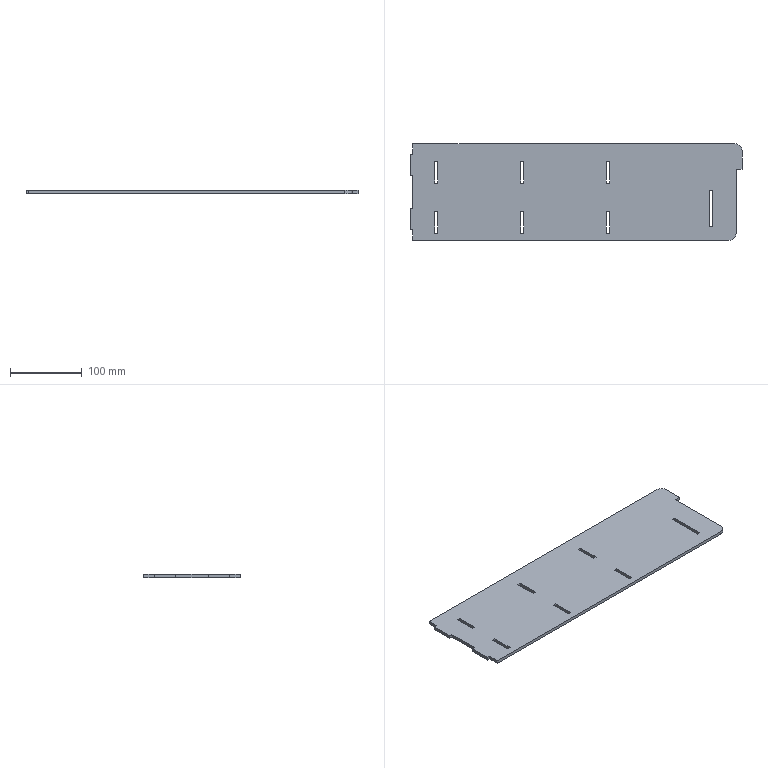Part | SolidWorks | features Fillet 1, FlatPattern 1, SMBaseFlange 1, SheetMetal 1 | 1 solid | 46 faces | box 464 x 135 x 4.5 mm | volume 271971 mm3 | plane 44 | cylinder 2 | commonest cylinder face diameters 20 x2
STEP:
#1=CARTESIAN_POINT('',(-230.,-90.,4.5));
#2=VERTEX_POINT('',#1);
#3=CARTESIAN_POINT('',(211.7,-90.,4.5));
#4=VERTEX_POINT('',#3);
#5=CARTESIAN_POINT('',(-230.,-90.,4.5));
#6=DIRECTION('',(1.,0.,0.));
#7=VECTOR('',#6,1000.);
#8=LINE('',#5,#7);
#9=EDGE_CURVE('',#2,#4,#8,.T.);
#10=ORIENTED_EDGE('',*,*,#9,.T.);
#11=CARTESIAN_POINT('',(221.7,-80.,4.5));
#12=VERTEX_POINT('',#11);
#13=CARTESIAN_POINT('',(211.7,-80.,4.5));
#14=DIRECTION('',(0.,0.,1.));
#15=DIRECTION('',(1.,0.,0.));
#16=AXIS2_PLACEMENT_3D('',#13,#14,#15);
#17=CIRCLE('',#16,10.);
#18=EDGE_CURVE('',#4,#12,#17,.T.);
#19=ORIENTED_EDGE('',*,*,#18,.T.);
#20=CARTESIAN_POINT('',(221.7,9.3,4.5));
#21=VERTEX_POINT('',#20);
#22=CARTESIAN_POINT('',(221.7,9.3,4.5));
#23=DIRECTION('',(0.,1.,0.));
#24=VECTOR('',#23,1000.);
#25=LINE('',#22,#24);
#26=EDGE_CURVE('',#12,#21,#25,.T.);
#27=ORIENTED_EDGE('',*,*,#26,.T.);
#28=CARTESIAN_POINT('',(230.,9.3,4.5));
#29=VERTEX_POINT('',#28);
#30=CARTESIAN_POINT('',(221.7,9.3,4.5));
#31=DIRECTION('',(1.,0.,0.));
#32=VECTOR('',#31,1000.);
#33=LINE('',#30,#32);
#34=EDGE_CURVE('',#21,#29,#33,.T.);
#35=ORIENTED_EDGE('',*,*,#34,.T.);
#36=CARTESIAN_POINT('',(230.,35.,4.5));
#37=VERTEX_POINT('',#36);
#38=CARTESIAN_POINT('',(230.,9.3,4.5));
#39=DIRECTION('',(0.,1.,0.));
#40=VECTOR('',#39,1000.);
#41=LINE('',#38,#40);
#42=EDGE_CURVE('',#29,#37,#41,.T.);
#43=ORIENTED_EDGE('',*,*,#42,.T.);
#44=CARTESIAN_POINT('',(220.,45.,4.5));
#45=VERTEX_POINT('',#44);
#46=CARTESIAN_POINT('',(220.,35.,4.5));
#47=DIRECTION('',(0.,0.,1.));
#48=DIRECTION('',(1.,0.,0.));
#49=AXIS2_PLACEMENT_3D('',#46,#47,#48);
#50=CIRCLE('',#49,10.);
#51=EDGE_CURVE('',#37,#45,#50,.T.);
#52=ORIENTED_EDGE('',*,*,#51,.T.);
#53=CARTESIAN_POINT('',(-230.,45.,4.5));
#54=VERTEX_POINT('',#53);
#55=CARTESIAN_POINT('',(-230.,45.,4.5));
#56=DIRECTION('',(-1.,0.,0.));
#57=VECTOR('',#56,1000.);
#58=LINE('',#55,#57);
#59=EDGE_CURVE('',#45,#54,#58,.T.);
#60=ORIENTED_EDGE('',*,*,#59,.T.);
#61=CARTESIAN_POINT('',(-230.,30.,4.5));
#62=VERTEX_POINT('',#61);
#63=CARTESIAN_POINT('',(-230.,45.,4.5));
#64=DIRECTION('',(0.,-1.,0.));
#65=VECTOR('',#64,1000.);
#66=LINE('',#63,#65);
#67=EDGE_CURVE('',#54,#62,#66,.T.);
#68=ORIENTED_EDGE('',*,*,#67,.T.);
#69=CARTESIAN_POINT('',(-234.,30.,4.5));
#70=VERTEX_POINT('',#69);
#71=CARTESIAN_POINT('',(-234.,30.,4.5));
#72=DIRECTION('',(-1.,0.,0.));
#73=VECTOR('',#72,1000.);
#74=LINE('',#71,#73);
#75=EDGE_CURVE('',#62,#70,#74,.T.);
#76=ORIENTED_EDGE('',*,*,#75,.T.);
#77=CARTESIAN_POINT('',(-234.,0.,4.5));
#78=VERTEX_POINT('',#77);
#79=CARTESIAN_POINT('',(-234.,0.,4.5));
#80=DIRECTION('',(0.,-1.,0.));
#81=VECTOR('',#80,1000.);
#82=LINE('',#79,#81);
#83=EDGE_CURVE('',#70,#78,#82,.T.);
#84=ORIENTED_EDGE('',*,*,#83,.T.);
#85=CARTESIAN_POINT('',(-230.,0.,4.5));
#86=VERTEX_POINT('',#85);
#87=CARTESIAN_POINT('',(-230.,0.,4.5));
#88=DIRECTION('',(1.,0.,0.));
#89=VECTOR('',#88,1000.);
#90=LINE('',#87,#89);
#91=EDGE_CURVE('',#78,#86,#90,.T.);
#92=ORIENTED_EDGE('',*,*,#91,.T.);
#93=CARTESIAN_POINT('',(-230.,-45.,4.5));
#94=VERTEX_POINT('',#93);
#95=CARTESIAN_POINT('',(-230.,0.,4.5));
#96=DIRECTION('',(0.,-1.,0.));
#97=VECTOR('',#96,1000.);
#98=LINE('',#95,#97);
#99=EDGE_CURVE('',#86,#94,#98,.T.);
#100=ORIENTED_EDGE('',*,*,#99,.T.);
#101=CARTESIAN_POINT('',(-234.,-45.,4.5));
#102=VERTEX_POINT('',#101);
#103=CARTESIAN_POINT('',(-234.,-45.,4.5));
#104=DIRECTION('',(-1.,0.,0.));
#105=VECTOR('',#104,1000.);
#106=LINE('',#103,#105);
#107=EDGE_CURVE('',#94,#102,#106,.T.);
#108=ORIENTED_EDGE('',*,*,#107,.T.);
#109=CARTESIAN_POINT('',(-234.,-75.,4.5));
#110=VERTEX_POINT('',#109);
#111=CARTESIAN_POINT('',(-234.,-75.,4.5));
#112=DIRECTION('',(0.,-1.,0.));
#113=VECTOR('',#112,1000.);
#114=LINE('',#111,#113);
#115=EDGE_CURVE('',#102,#110,#114,.T.);
#116=ORIENTED_EDGE('',*,*,#115,.T.);
#117=CARTESIAN_POINT('',(-230.,-75.,4.5));
#118=VERTEX_POINT('',#117);
#119=CARTESIAN_POINT('',(-230.,-75.,4.5));
#120=DIRECTION('',(1.,0.,0.));
#121=VECTOR('',#120,1000.);
#122=LINE('',#119,#121);
#123=EDGE_CURVE('',#110,#118,#122,.T.);
#124=ORIENTED_EDGE('',*,*,#123,.T.);
#125=CARTESIAN_POINT('',(-230.,-75.,4.5));
#126=DIRECTION('',(0.,-1.,0.));
#127=VECTOR('',#126,1000.);
#128=LINE('',#125,#127);
#129=EDGE_CURVE('',#118,#2,#128,.T.);
#130=ORIENTED_EDGE('',*,*,#129,.T.);
#131=EDGE_LOOP('',(#10,#19,#27,#35,#43,#52,#60,#68,#76,#84,#92,#100,#108,#116,#124,#130));
#132=FACE_OUTER_BOUND('',#131,.T.);
#133=CARTESIAN_POINT('',(189.,-20.7,4.5));
#134=VERTEX_POINT('',#133);
#135=CARTESIAN_POINT('',(184.5,-20.7,4.5));
#136=VERTEX_POINT('',#135);
#137=CARTESIAN_POINT('',(189.,-20.7,4.5));
#138=DIRECTION('',(-1.,0.,0.));
#139=VECTOR('',#138,1000.);
#140=LINE('',#137,#139);
#141=EDGE_CURVE('',#134,#136,#140,.T.);
#142=ORIENTED_EDGE('',*,*,#141,.F.);
#143=CARTESIAN_POINT('',(189.,-70.7,4.5));
#144=VERTEX_POINT('',#143);
#145=CARTESIAN_POINT('',(189.,-70.7,4.5));
#146=DIRECTION('',(0.,1.,0.));
#147=VECTOR('',#146,1000.);
#148=LINE('',#145,#147);
#149=EDGE_CURVE('',#144,#134,#148,.T.);
#150=ORIENTED_EDGE('',*,*,#149,.F.);
#151=CARTESIAN_POINT('',(184.5,-70.7,4.5));
#152=VERTEX_POINT('',#151);
#153=CARTESIAN_POINT('',(189.,-70.7,4.5));
#154=DIRECTION('',(1.,0.,0.));
#155=VECTOR('',#154,1000.);
#156=LINE('',#153,#155);
#157=EDGE_CURVE('',#152,#144,#156,.T.);
#158=ORIENTED_EDGE('',*,*,#157,.F.);
#159=CARTESIAN_POINT('',(184.5,-70.7,4.5));
#160=DIRECTION('',(0.,-1.,0.));
#161=VECTOR('',#160,1000.);
#162=LINE('',#159,#161);
#163=EDGE_CURVE('',#136,#152,#162,.T.);
#164=ORIENTED_EDGE('',*,*,#163,.F.);
#165=EDGE_LOOP('',(#142,#150,#158,#164));
#166=FACE_BOUND('',#165,.T.);
#167=CARTESIAN_POINT('',(45.,-50.,4.5));
#168=VERTEX_POINT('',#167);
#169=CARTESIAN_POINT('',(40.5,-50.,4.5));
#170=VERTEX_POINT('',#169);
#171=CARTESIAN_POINT('',(45.,-50.,4.5));
#172=DIRECTION('',(-1.,0.,0.));
#173=VECTOR('',#172,1000.);
#174=LINE('',#171,#173);
#175=EDGE_CURVE('',#168,#170,#174,.T.);
#176=ORIENTED_EDGE('',*,*,#175,.F.);
#177=CARTESIAN_POINT('',(45.,-80.,4.5));
#178=VERTEX_POINT('',#177);
#179=CARTESIAN_POINT('',(45.,-80.,4.5));
#180=DIRECTION('',(0.,1.,0.));
#181=VECTOR('',#180,1000.);
#182=LINE('',#179,#181);
#183=EDGE_CURVE('',#178,#168,#182,.T.);
#184=ORIENTED_EDGE('',*,*,#183,.F.);
#185=CARTESIAN_POINT('',(40.5,-80.,4.5));
#186=VERTEX_POINT('',#185);
#187=CARTESIAN_POINT('',(45.,-80.,4.5));
#188=DIRECTION('',(1.,0.,0.));
#189=VECTOR('',#188,1000.);
#190=LINE('',#187,#189);
#191=EDGE_CURVE('',#186,#178,#190,.T.);
#192=ORIENTED_EDGE('',*,*,#191,.F.);
#193=CARTESIAN_POINT('',(40.5,-80.,4.5));
#194=DIRECTION('',(0.,-1.,0.));
#195=VECTOR('',#194,1000.);
#196=LINE('',#193,#195);
#197=EDGE_CURVE('',#170,#186,#196,.T.);
#198=ORIENTED_EDGE('',*,*,#197,.F.);
#199=EDGE_LOOP('',(#176,#184,#192,#198));
#200=FACE_BOUND('',#199,.T.);
#201=CARTESIAN_POINT('',(45.,20.,4.5));
#202=VERTEX_POINT('',#201);
#203=CARTESIAN_POINT('',(40.5,20.,4.5));
#204=VERTEX_POINT('',#203);
#205=CARTESIAN_POINT('',(45.,20.,4.5));
#206=DIRECTION('',(-1.,0.,0.));
#207=VECTOR('',#206,1000.);
#208=LINE('',#205,#207);
#209=EDGE_CURVE('',#202,#204,#208,.T.);
#210=ORIENTED_EDGE('',*,*,#209,.F.);
#211=CARTESIAN_POINT('',(45.,-10.,4.5));
#212=VERTEX_POINT('',#211);
#213=CARTESIAN_POINT('',(45.,-10.,4.5));
#214=DIRECTION('',(0.,1.,0.));
#215=VECTOR('',#214,1000.);
#216=LINE('',#213,#215);
#217=EDGE_CURVE('',#212,#202,#216,.T.);
#218=ORIENTED_EDGE('',*,*,#217,.F.);
#219=CARTESIAN_POINT('',(40.5,-10.,4.5));
#220=VERTEX_POINT('',#219);
#221=CARTESIAN_POINT('',(45.,-10.,4.5));
#222=DIRECTION('',(1.,0.,0.));
#223=VECTOR('',#222,1000.);
#224=LINE('',#221,#223);
#225=EDGE_CURVE('',#220,#212,#224,.T.);
#226=ORIENTED_EDGE('',*,*,#225,.F.);
#227=CARTESIAN_POINT('',(40.5,-10.,4.5));
#228=DIRECTION('',(0.,-1.,0.));
#229=VECTOR('',#228,1000.);
#230=LINE('',#227,#229);
#231=EDGE_CURVE('',#204,#220,#230,.T.);
#232=ORIENTED_EDGE('',*,*,#231,.F.);
#233=EDGE_LOOP('',(#210,#218,#226,#232));
#234=FACE_BOUND('',#233,.T.);
#235=CARTESIAN_POINT('',(-75.,20.,4.5));
#236=VERTEX_POINT('',#235);
#237=CARTESIAN_POINT('',(-79.5,20.,4.5));
#238=VERTEX_POINT('',#237);
#239=CARTESIAN_POINT('',(-75.,20.,4.5));
#240=DIRECTION('',(-1.,0.,0.));
#241=VECTOR('',#240,1000.);
#242=LINE('',#239,#241);
#243=EDGE_CURVE('',#236,#238,#242,.T.);
#244=ORIENTED_EDGE('',*,*,#243,.F.);
#245=CARTESIAN_POINT('',(-75.,-10.,4.5));
#246=VERTEX_POINT('',#245);
#247=CARTESIAN_POINT('',(-75.,20.,4.5));
#248=DIRECTION('',(0.,1.,0.));
#249=VECTOR('',#248,1000.);
#250=LINE('',#247,#249);
#251=EDGE_CURVE('',#246,#236,#250,.T.);
#252=ORIENTED_EDGE('',*,*,#251,.F.);
#253=CARTESIAN_POINT('',(-79.5,-10.,4.5));
#254=VERTEX_POINT('',#253);
#255=CARTESIAN_POINT('',(-75.,-10.,4.5));
#256=DIRECTION('',(1.,0.,0.));
#257=VECTOR('',#256,1000.);
#258=LINE('',#255,#257);
#259=EDGE_CURVE('',#254,#246,#258,.T.);
#260=ORIENTED_EDGE('',*,*,#259,.F.);
#261=CARTESIAN_POINT('',(-79.5,20.,4.5));
#262=DIRECTION('',(0.,-1.,0.));
#263=VECTOR('',#262,1000.);
#264=LINE('',#261,#263);
#265=EDGE_CURVE('',#238,#254,#264,.T.);
#266=ORIENTED_EDGE('',*,*,#265,.F.);
#267=EDGE_LOOP('',(#244,#252,#260,#266));
#268=FACE_BOUND('',#267,.T.);
#269=CARTESIAN_POINT('',(-75.,-50.,4.5));
#270=VERTEX_POINT('',#269);
#271=CARTESIAN_POINT('',(-79.5,-50.,4.5));
#272=VERTEX_POINT('',#271);
#273=CARTESIAN_POINT('',(-75.,-50.,4.5));
#274=DIRECTION('',(-1.,0.,0.));
#275=VECTOR('',#274,1000.);
#276=LINE('',#273,#275);
#277=EDGE_CURVE('',#270,#272,#276,.T.);
#278=ORIENTED_EDGE('',*,*,#277,.F.);
#279=CARTESIAN_POINT('',(-75.,-80.,4.5));
#280=VERTEX_POINT('',#279);
#281=CARTESIAN_POINT('',(-75.,-80.,4.5));
#282=DIRECTION('',(0.,1.,0.));
#283=VECTOR('',#282,1000.);
#284=LINE('',#281,#283);
#285=EDGE_CURVE('',#280,#270,#284,.T.);
#286=ORIENTED_EDGE('',*,*,#285,.F.);
#287=CARTESIAN_POINT('',(-79.5,-80.,4.5));
#288=VERTEX_POINT('',#287);
#289=CARTESIAN_POINT('',(-75.,-80.,4.5));
#290=DIRECTION('',(1.,0.,0.));
#291=VECTOR('',#290,1000.);
#292=LINE('',#289,#291);
#293=EDGE_CURVE('',#288,#280,#292,.T.);
#294=ORIENTED_EDGE('',*,*,#293,.F.);
#295=CARTESIAN_POINT('',(-79.5,-80.,4.5));
#296=DIRECTION('',(0.,-1.,0.));
#297=VECTOR('',#296,1000.);
#298=LINE('',#295,#297);
#299=EDGE_CURVE('',#272,#288,#298,.T.);
#300=ORIENTED_EDGE('',*,*,#299,.F.);
#301=EDGE_LOOP('',(#278,#286,#294,#300));
#302=FACE_BOUND('',#301,.T.);
#303=CARTESIAN_POINT('',(-195.,20.,4.5));
#304=VERTEX_POINT('',#303);
#305=CARTESIAN_POINT('',(-199.5,20.,4.5));
#306=VERTEX_POINT('',#305);
#307=CARTESIAN_POINT('',(-195.,20.,4.5));
#308=DIRECTION('',(-1.,0.,0.));
#309=VECTOR('',#308,1000.);
#310=LINE('',#307,#309);
#311=EDGE_CURVE('',#304,#306,#310,.T.);
#312=ORIENTED_EDGE('',*,*,#311,.F.);
#313=CARTESIAN_POINT('',(-195.,-10.,4.5));
#314=VERTEX_POINT('',#313);
#315=CARTESIAN_POINT('',(-195.,20.,4.5));
#316=DIRECTION('',(0.,1.,0.));
#317=VECTOR('',#316,1000.);
#318=LINE('',#315,#317);
#319=EDGE_CURVE('',#314,#304,#318,.T.);
#320=ORIENTED_EDGE('',*,*,#319,.F.);
#321=CARTESIAN_POINT('',(-199.5,-10.,4.5));
#322=VERTEX_POINT('',#321);
#323=CARTESIAN_POINT('',(-195.,-10.,4.5));
#324=DIRECTION('',(1.,0.,0.));
#325=VECTOR('',#324,1000.);
#326=LINE('',#323,#325);
#327=EDGE_CURVE('',#322,#314,#326,.T.);
#328=ORIENTED_EDGE('',*,*,#327,.F.);
#329=CARTESIAN_POINT('',(-199.5,20.,4.5));
#330=DIRECTION('',(0.,-1.,0.));
#331=VECTOR('',#330,1000.);
#332=LINE('',#329,#331);
#333=EDGE_CURVE('',#306,#322,#332,.T.);
#334=ORIENTED_EDGE('',*,*,#333,.F.);
#335=EDGE_LOOP('',(#312,#320,#328,#334));
#336=FACE_BOUND('',#335,.T.);
#337=CARTESIAN_POINT('',(-195.,-50.,4.5));
#338=VERTEX_POINT('',#337);
#339=CARTESIAN_POINT('',(-199.5,-50.,4.5));
#340=VERTEX_POINT('',#339);
#341=CARTESIAN_POINT('',(-195.,-50.,4.5));
#342=DIRECTION('',(-1.,0.,0.));
#343=VECTOR('',#342,1000.);
#344=LINE('',#341,#343);
#345=EDGE_CURVE('',#338,#340,#344,.T.);
#346=ORIENTED_EDGE('',*,*,#345,.F.);
#347=CARTESIAN_POINT('',(-195.,-80.,4.5));
#348=VERTEX_POINT('',#347);
#349=CARTESIAN_POINT('',(-195.,-80.,4.5));
#350=DIRECTION('',(0.,1.,0.));
#351=VECTOR('',#350,1000.);
#352=LINE('',#349,#351);
#353=EDGE_CURVE('',#348,#338,#352,.T.);
#354=ORIENTED_EDGE('',*,*,#353,.F.);
#355=CARTESIAN_POINT('',(-199.5,-80.,4.5));
#356=VERTEX_POINT('',#355);
#357=CARTESIAN_POINT('',(-195.,-80.,4.5));
#358=DIRECTION('',(1.,0.,0.));
#359=VECTOR('',#358,1000.);
#360=LINE('',#357,#359);
#361=EDGE_CURVE('',#356,#348,#360,.T.);
#362=ORIENTED_EDGE('',*,*,#361,.F.);
#363=CARTESIAN_POINT('',(-199.5,-80.,4.5));
#364=DIRECTION('',(0.,-1.,0.));
#365=VECTOR('',#364,1000.);
#366=LINE('',#363,#365);
#367=EDGE_CURVE('',#340,#356,#366,.T.);
#368=ORIENTED_EDGE('',*,*,#367,.F.);
#369=EDGE_LOOP('',(#346,#354,#362,#368));
#370=FACE_BOUND('',#369,.T.);
#371=CARTESIAN_POINT('',(0.,0.,4.5));
#372=DIRECTION('',(0.,0.,1.));
#373=DIRECTION('',(1.,0.,0.));
#374=AXIS2_PLACEMENT_3D('',#371,#372,#373);
#375=PLANE('',#374);
#376=ADVANCED_FACE('',(#132,#166,#200,#234,#268,#302,#336,#370),#375,.T.);
#377=CARTESIAN_POINT('',(-195.,-10.,0.));
#378=VERTEX_POINT('',#377);
#379=CARTESIAN_POINT('',(-195.,20.,0.));
#380=VERTEX_POINT('',#379);
#381=CARTESIAN_POINT('',(-195.,20.,0.));
#382=DIRECTION('',(0.,1.,0.));
#383=VECTOR('',#382,1000.);
#384=LINE('',#381,#383);
#385=EDGE_CURVE('',#378,#380,#384,.T.);
#386=ORIENTED_EDGE('',*,*,#385,.T.);
#387=CARTESIAN_POINT('',(-199.5,20.,0.));
#388=VERTEX_POINT('',#387);
#389=CARTESIAN_POINT('',(-195.,20.,0.));
#390=DIRECTION('',(-1.,0.,0.));
#391=VECTOR('',#390,1000.);
#392=LINE('',#389,#391);
#393=EDGE_CURVE('',#380,#388,#392,.T.);
#394=ORIENTED_EDGE('',*,*,#393,.T.);
#395=CARTESIAN_POINT('',(-199.5,-10.,0.));
#396=VERTEX_POINT('',#395);
#397=CARTESIAN_POINT('',(-199.5,20.,0.));
#398=DIRECTION('',(0.,-1.,0.));
#399=VECTOR('',#398,1000.);
#400=LINE('',#397,#399);
#401=EDGE_CURVE('',#388,#396,#400,.T.);
#402=ORIENTED_EDGE('',*,*,#401,.T.);
#403=CARTESIAN_POINT('',(-195.,-10.,0.));
#404=DIRECTION('',(1.,0.,0.));
#405=VECTOR('',#404,1000.);
#406=LINE('',#403,#405);
#407=EDGE_CURVE('',#396,#378,#406,.T.);
#408=ORIENTED_EDGE('',*,*,#407,.T.);
#409=EDGE_LOOP('',(#386,#394,#402,#408));
#410=FACE_BOUND('',#409,.T.);
#411=CARTESIAN_POINT('',(-75.,-10.,0.));
#412=VERTEX_POINT('',#411);
#413=CARTESIAN_POINT('',(-75.,20.,0.));
#414=VERTEX_POINT('',#413);
#415=CARTESIAN_POINT('',(-75.,20.,0.));
#416=DIRECTION('',(0.,1.,0.));
#417=VECTOR('',#416,1000.);
#418=LINE('',#415,#417);
#419=EDGE_CURVE('',#412,#414,#418,.T.);
#420=ORIENTED_EDGE('',*,*,#419,.T.);
#421=CARTESIAN_POINT('',(-79.5,20.,0.));
#422=VERTEX_POINT('',#421);
#423=CARTESIAN_POINT('',(-75.,20.,0.));
#424=DIRECTION('',(-1.,0.,0.));
#425=VECTOR('',#424,1000.);
#426=LINE('',#423,#425);
#427=EDGE_CURVE('',#414,#422,#426,.T.);
#428=ORIENTED_EDGE('',*,*,#427,.T.);
#429=CARTESIAN_POINT('',(-79.5,-10.,0.));
#430=VERTEX_POINT('',#429);
#431=CARTESIAN_POINT('',(-79.5,20.,0.));
#432=DIRECTION('',(0.,-1.,0.));
#433=VECTOR('',#432,1000.);
#434=LINE('',#431,#433);
#435=EDGE_CURVE('',#422,#430,#434,.T.);
#436=ORIENTED_EDGE('',*,*,#435,.T.);
#437=CARTESIAN_POINT('',(-75.,-10.,0.));
#438=DIRECTION('',(1.,0.,0.));
#439=VECTOR('',#438,1000.);
#440=LINE('',#437,#439);
#441=EDGE_CURVE('',#430,#412,#440,.T.);
#442=ORIENTED_EDGE('',*,*,#441,.T.);
#443=EDGE_LOOP('',(#420,#428,#436,#442));
#444=FACE_BOUND('',#443,.T.);
#445=CARTESIAN_POINT('',(45.,-80.,0.));
#446=VERTEX_POINT('',#445);
#447=CARTESIAN_POINT('',(45.,-50.,0.));
#448=VERTEX_POINT('',#447);
#449=CARTESIAN_POINT('',(45.,-80.,0.));
#450=DIRECTION('',(0.,1.,0.));
#451=VECTOR('',#450,1000.);
#452=LINE('',#449,#451);
#453=EDGE_CURVE('',#446,#448,#452,.T.);
#454=ORIENTED_EDGE('',*,*,#453,.T.);
#455=CARTESIAN_POINT('',(40.5,-50.,0.));
#456=VERTEX_POINT('',#455);
#457=CARTESIAN_POINT('',(45.,-50.,0.));
#458=DIRECTION('',(-1.,0.,0.));
#459=VECTOR('',#458,1000.);
#460=LINE('',#457,#459);
#461=EDGE_CURVE('',#448,#456,#460,.T.);
#462=ORIENTED_EDGE('',*,*,#461,.T.);
#463=CARTESIAN_POINT('',(40.5,-80.,0.));
#464=VERTEX_POINT('',#463);
#465=CARTESIAN_POINT('',(40.5,-80.,0.));
#466=DIRECTION('',(0.,-1.,0.));
#467=VECTOR('',#466,1000.);
#468=LINE('',#465,#467);
#469=EDGE_CURVE('',#456,#464,#468,.T.);
#470=ORIENTED_EDGE('',*,*,#469,.T.);
#471=CARTESIAN_POINT('',(45.,-80.,0.));
#472=DIRECTION('',(1.,0.,0.));
#473=VECTOR('',#472,1000.);
#474=LINE('',#471,#473);
#475=EDGE_CURVE('',#464,#446,#474,.T.);
#476=ORIENTED_EDGE('',*,*,#475,.T.);
#477=EDGE_LOOP('',(#454,#462,#470,#476));
#478=FACE_BOUND('',#477,.T.);
#479=CARTESIAN_POINT('',(221.7,-80.,0.));
#480=VERTEX_POINT('',#479);
#481=CARTESIAN_POINT('',(221.7,9.3,0.));
#482=VERTEX_POINT('',#481);
#483=CARTESIAN_POINT('',(221.7,9.3,0.));
#484=DIRECTION('',(0.,1.,0.));
#485=VECTOR('',#484,1000.);
#486=LINE('',#483,#485);
#487=EDGE_CURVE('',#480,#482,#486,.T.);
#488=ORIENTED_EDGE('',*,*,#487,.F.);
#489=CARTESIAN_POINT('',(211.7,-90.,0.));
#490=VERTEX_POINT('',#489);
#491=CARTESIAN_POINT('',(211.7,-80.,0.));
#492=DIRECTION('',(0.,0.,-1.));
#493=DIRECTION('',(1.,0.,0.));
#494=AXIS2_PLACEMENT_3D('',#491,#492,#493);
#495=CIRCLE('',#494,10.);
#496=EDGE_CURVE('',#480,#490,#495,.T.);
#497=ORIENTED_EDGE('',*,*,#496,.T.);
#498=CARTESIAN_POINT('',(-230.,-90.,0.));
#499=VERTEX_POINT('',#498);
#500=CARTESIAN_POINT('',(-230.,-90.,0.));
#501=DIRECTION('',(1.,0.,0.));
#502=VECTOR('',#501,1000.);
#503=LINE('',#500,#502);
#504=EDGE_CURVE('',#499,#490,#503,.T.);
#505=ORIENTED_EDGE('',*,*,#504,.F.);
#506=CARTESIAN_POINT('',(-230.,-75.,0.));
#507=VERTEX_POINT('',#506);
#508=CARTESIAN_POINT('',(-230.,-75.,0.));
#509=DIRECTION('',(0.,-1.,0.));
#510=VECTOR('',#509,1000.);
#511=LINE('',#508,#510);
#512=EDGE_CURVE('',#507,#499,#511,.T.);
#513=ORIENTED_EDGE('',*,*,#512,.F.);
#514=CARTESIAN_POINT('',(-234.,-75.,0.));
#515=VERTEX_POINT('',#514);
#516=CARTESIAN_POINT('',(-230.,-75.,0.));
#517=DIRECTION('',(1.,0.,0.));
#518=VECTOR('',#517,1000.);
#519=LINE('',#516,#518);
#520=EDGE_CURVE('',#515,#507,#519,.T.);
#521=ORIENTED_EDGE('',*,*,#520,.F.);
#522=CARTESIAN_POINT('',(-234.,-45.,0.));
#523=VERTEX_POINT('',#522);
#524=CARTESIAN_POINT('',(-234.,-75.,0.));
#525=DIRECTION('',(0.,-1.,0.));
#526=VECTOR('',#525,1000.);
#527=LINE('',#524,#526);
#528=EDGE_CURVE('',#523,#515,#527,.T.);
#529=ORIENTED_EDGE('',*,*,#528,.F.);
#530=CARTESIAN_POINT('',(-230.,-45.,0.));
#531=VERTEX_POINT('',#530);
#532=CARTESIAN_POINT('',(-234.,-45.,0.));
#533=DIRECTION('',(-1.,0.,0.));
#534=VECTOR('',#533,1000.);
#535=LINE('',#532,#534);
#536=EDGE_CURVE('',#531,#523,#535,.T.);
#537=ORIENTED_EDGE('',*,*,#536,.F.);
#538=CARTESIAN_POINT('',(-230.,0.,0.));
#539=VERTEX_POINT('',#538);
#540=CARTESIAN_POINT('',(-230.,0.,0.));
#541=DIRECTION('',(0.,-1.,0.));
#542=VECTOR('',#541,1000.);
#543=LINE('',#540,#542);
#544=EDGE_CURVE('',#539,#531,#543,.T.);
#545=ORIENTED_EDGE('',*,*,#544,.F.);
#546=CARTESIAN_POINT('',(-234.,0.,0.));
#547=VERTEX_POINT('',#546);
#548=CARTESIAN_POINT('',(-230.,0.,0.));
#549=DIRECTION('',(1.,0.,0.));
#550=VECTOR('',#549,1000.);
#551=LINE('',#548,#550);
#552=EDGE_CURVE('',#547,#539,#551,.T.);
#553=ORIENTED_EDGE('',*,*,#552,.F.);
#554=CARTESIAN_POINT('',(-234.,30.,0.));
#555=VERTEX_POINT('',#554);
#556=CARTESIAN_POINT('',(-234.,0.,0.));
#557=DIRECTION('',(0.,-1.,0.));
#558=VECTOR('',#557,1000.);
#559=LINE('',#556,#558);
#560=EDGE_CURVE('',#555,#547,#559,.T.);
#561=ORIENTED_EDGE('',*,*,#560,.F.);
#562=CARTESIAN_POINT('',(-230.,30.,0.));
#563=VERTEX_POINT('',#562);
#564=CARTESIAN_POINT('',(-234.,30.,0.));
#565=DIRECTION('',(-1.,0.,0.));
#566=VECTOR('',#565,1000.);
#567=LINE('',#564,#566);
#568=EDGE_CURVE('',#563,#555,#567,.T.);
#569=ORIENTED_EDGE('',*,*,#568,.F.);
#570=CARTESIAN_POINT('',(-230.,45.,0.));
#571=VERTEX_POINT('',#570);
#572=CARTESIAN_POINT('',(-230.,45.,0.));
#573=DIRECTION('',(0.,-1.,0.));
#574=VECTOR('',#573,1000.);
#575=LINE('',#572,#574);
#576=EDGE_CURVE('',#571,#563,#575,.T.);
#577=ORIENTED_EDGE('',*,*,#576,.F.);
#578=CARTESIAN_POINT('',(220.,45.,0.));
#579=VERTEX_POINT('',#578);
#580=CARTESIAN_POINT('',(-230.,45.,0.));
#581=DIRECTION('',(-1.,0.,0.));
#582=VECTOR('',#581,1000.);
#583=LINE('',#580,#582);
#584=EDGE_CURVE('',#579,#571,#583,.T.);
#585=ORIENTED_EDGE('',*,*,#584,.F.);
#586=CARTESIAN_POINT('',(230.,35.,0.));
#587=VERTEX_POINT('',#586);
#588=CARTESIAN_POINT('',(220.,35.,0.));
#589=DIRECTION('',(0.,0.,-1.));
#590=DIRECTION('',(1.,0.,0.));
#591=AXIS2_PLACEMENT_3D('',#588,#589,#590);
#592=CIRCLE('',#591,10.);
#593=EDGE_CURVE('',#579,#587,#592,.T.);
#594=ORIENTED_EDGE('',*,*,#593,.T.);
#595=CARTESIAN_POINT('',(230.,9.3,0.));
#596=VERTEX_POINT('',#595);
#597=CARTESIAN_POINT('',(230.,9.3,0.));
#598=DIRECTION('',(0.,1.,0.));
#599=VECTOR('',#598,1000.);
#600=LINE('',#597,#599);
#601=EDGE_CURVE('',#596,#587,#600,.T.);
#602=ORIENTED_EDGE('',*,*,#601,.F.);
#603=CARTESIAN_POINT('',(221.7,9.3,0.));
#604=DIRECTION('',(1.,0.,0.));
#605=VECTOR('',#604,1000.);
#606=LINE('',#603,#605);
#607=EDGE_CURVE('',#482,#596,#606,.T.);
#608=ORIENTED_EDGE('',*,*,#607,.F.);
#609=EDGE_LOOP('',(#488,#497,#505,#513,#521,#529,#537,#545,#553,#561,#569,#577,#585,#594,#602,#608));
#610=FACE_OUTER_BOUND('',#609,.T.);
#611=CARTESIAN_POINT('',(189.,-70.7,0.));
#612=VERTEX_POINT('',#611);
#613=CARTESIAN_POINT('',(189.,-20.7,0.));
#614=VERTEX_POINT('',#613);
#615=CARTESIAN_POINT('',(189.,-70.7,0.));
#616=DIRECTION('',(0.,1.,0.));
#617=VECTOR('',#616,1000.);
#618=LINE('',#615,#617);
#619=EDGE_CURVE('',#612,#614,#618,.T.);
#620=ORIENTED_EDGE('',*,*,#619,.T.);
#621=CARTESIAN_POINT('',(184.5,-20.7,0.));
#622=VERTEX_POINT('',#621);
#623=CARTESIAN_POINT('',(189.,-20.7,0.));
#624=DIRECTION('',(-1.,0.,0.));
#625=VECTOR('',#624,1000.);
#626=LINE('',#623,#625);
#627=EDGE_CURVE('',#614,#622,#626,.T.);
#628=ORIENTED_EDGE('',*,*,#627,.T.);
#629=CARTESIAN_POINT('',(184.5,-70.7,0.));
#630=VERTEX_POINT('',#629);
#631=CARTESIAN_POINT('',(184.5,-70.7,0.));
#632=DIRECTION('',(0.,-1.,0.));
#633=VECTOR('',#632,1000.);
#634=LINE('',#631,#633);
#635=EDGE_CURVE('',#622,#630,#634,.T.);
#636=ORIENTED_EDGE('',*,*,#635,.T.);
#637=CARTESIAN_POINT('',(189.,-70.7,0.));
#638=DIRECTION('',(1.,0.,0.));
#639=VECTOR('',#638,1000.);
#640=LINE('',#637,#639);
#641=EDGE_CURVE('',#630,#612,#640,.T.);
#642=ORIENTED_EDGE('',*,*,#641,.T.);
#643=EDGE_LOOP('',(#620,#628,#636,#642));
#644=FACE_BOUND('',#643,.T.);
#645=CARTESIAN_POINT('',(45.,-10.,0.));
#646=VERTEX_POINT('',#645);
#647=CARTESIAN_POINT('',(45.,20.,0.));
#648=VERTEX_POINT('',#647);
#649=CARTESIAN_POINT('',(45.,-10.,0.));
#650=DIRECTION('',(0.,1.,0.));
#651=VECTOR('',#650,1000.);
#652=LINE('',#649,#651);
#653=EDGE_CURVE('',#646,#648,#652,.T.);
#654=ORIENTED_EDGE('',*,*,#653,.T.);
#655=CARTESIAN_POINT('',(40.5,20.,0.));
#656=VERTEX_POINT('',#655);
#657=CARTESIAN_POINT('',(45.,20.,0.));
#658=DIRECTION('',(-1.,0.,0.));
#659=VECTOR('',#658,1000.);
#660=LINE('',#657,#659);
#661=EDGE_CURVE('',#648,#656,#660,.T.);
#662=ORIENTED_EDGE('',*,*,#661,.T.);
#663=CARTESIAN_POINT('',(40.5,-10.,0.));
#664=VERTEX_POINT('',#663);
#665=CARTESIAN_POINT('',(40.5,-10.,0.));
#666=DIRECTION('',(0.,-1.,0.));
#667=VECTOR('',#666,1000.);
#668=LINE('',#665,#667);
#669=EDGE_CURVE('',#656,#664,#668,.T.);
#670=ORIENTED_EDGE('',*,*,#669,.T.);
#671=CARTESIAN_POINT('',(45.,-10.,0.));
#672=DIRECTION('',(1.,0.,0.));
#673=VECTOR('',#672,1000.);
#674=LINE('',#671,#673);
#675=EDGE_CURVE('',#664,#646,#674,.T.);
#676=ORIENTED_EDGE('',*,*,#675,.T.);
#677=EDGE_LOOP('',(#654,#662,#670,#676));
#678=FACE_BOUND('',#677,.T.);
#679=CARTESIAN_POINT('',(-75.,-80.,0.));
#680=VERTEX_POINT('',#679);
#681=CARTESIAN_POINT('',(-75.,-50.,0.));
#682=VERTEX_POINT('',#681);
#683=CARTESIAN_POINT('',(-75.,-80.,0.));
#684=DIRECTION('',(0.,1.,0.));
#685=VECTOR('',#684,1000.);
#686=LINE('',#683,#685);
#687=EDGE_CURVE('',#680,#682,#686,.T.);
#688=ORIENTED_EDGE('',*,*,#687,.T.);
#689=CARTESIAN_POINT('',(-79.5,-50.,0.));
#690=VERTEX_POINT('',#689);
#691=CARTESIAN_POINT('',(-75.,-50.,0.));
#692=DIRECTION('',(-1.,0.,0.));
#693=VECTOR('',#692,1000.);
#694=LINE('',#691,#693);
#695=EDGE_CURVE('',#682,#690,#694,.T.);
#696=ORIENTED_EDGE('',*,*,#695,.T.);
#697=CARTESIAN_POINT('',(-79.5,-80.,0.));
#698=VERTEX_POINT('',#697);
#699=CARTESIAN_POINT('',(-79.5,-80.,0.));
#700=DIRECTION('',(0.,-1.,0.));
#701=VECTOR('',#700,1000.);
#702=LINE('',#699,#701);
#703=EDGE_CURVE('',#690,#698,#702,.T.);
#704=ORIENTED_EDGE('',*,*,#703,.T.);
#705=CARTESIAN_POINT('',(-75.,-80.,0.));
#706=DIRECTION('',(1.,0.,0.));
#707=VECTOR('',#706,1000.);
#708=LINE('',#705,#707);
#709=EDGE_CURVE('',#698,#680,#708,.T.);
#710=ORIENTED_EDGE('',*,*,#709,.T.);
#711=EDGE_LOOP('',(#688,#696,#704,#710));
#712=FACE_BOUND('',#711,.T.);
#713=CARTESIAN_POINT('',(-195.,-80.,0.));
#714=VERTEX_POINT('',#713);
#715=CARTESIAN_POINT('',(-195.,-50.,0.));
#716=VERTEX_POINT('',#715);
#717=CARTESIAN_POINT('',(-195.,-80.,0.));
#718=DIRECTION('',(0.,1.,0.));
#719=VECTOR('',#718,1000.);
#720=LINE('',#717,#719);
#721=EDGE_CURVE('',#714,#716,#720,.T.);
#722=ORIENTED_EDGE('',*,*,#721,.T.);
#723=CARTESIAN_POINT('',(-199.5,-50.,0.));
#724=VERTEX_POINT('',#723);
#725=CARTESIAN_POINT('',(-195.,-50.,0.));
#726=DIRECTION('',(-1.,0.,0.));
#727=VECTOR('',#726,1000.);
#728=LINE('',#725,#727);
#729=EDGE_CURVE('',#716,#724,#728,.T.);
#730=ORIENTED_EDGE('',*,*,#729,.T.);
#731=CARTESIAN_POINT('',(-199.5,-80.,0.));
#732=VERTEX_POINT('',#731);
#733=CARTESIAN_POINT('',(-199.5,-80.,0.));
#734=DIRECTION('',(0.,-1.,0.));
#735=VECTOR('',#734,1000.);
#736=LINE('',#733,#735);
#737=EDGE_CURVE('',#724,#732,#736,.T.);
#738=ORIENTED_EDGE('',*,*,#737,.T.);
#739=CARTESIAN_POINT('',(-195.,-80.,0.));
#740=DIRECTION('',(1.,0.,0.));
#741=VECTOR('',#740,1000.);
#742=LINE('',#739,#741);
#743=EDGE_CURVE('',#732,#714,#742,.T.);
#744=ORIENTED_EDGE('',*,*,#743,.T.);
#745=EDGE_LOOP('',(#722,#730,#738,#744));
#746=FACE_BOUND('',#745,.T.);
#747=CARTESIAN_POINT('',(0.,0.,0.));
#748=DIRECTION('',(0.,0.,1.));
#749=DIRECTION('',(1.,0.,0.));
#750=AXIS2_PLACEMENT_3D('',#747,#748,#749);
#751=PLANE('',#750);
#752=ADVANCED_FACE('',(#410,#444,#478,#610,#644,#678,#712,#746),#751,.F.);
#753=ORIENTED_EDGE('',*,*,#576,.T.);
#754=CARTESIAN_POINT('',(-230.,30.,4.5));
#755=DIRECTION('',(0.,0.,-1.));
#756=VECTOR('',#755,1000.);
#757=LINE('',#754,#756);
#758=EDGE_CURVE('',#62,#563,#757,.T.);
#759=ORIENTED_EDGE('',*,*,#758,.F.);
#760=ORIENTED_EDGE('',*,*,#67,.F.);
#761=CARTESIAN_POINT('',(-230.,45.,4.5));
#762=DIRECTION('',(0.,0.,-1.));
#763=VECTOR('',#762,1000.);
#764=LINE('',#761,#763);
#765=EDGE_CURVE('',#54,#571,#764,.T.);
#766=ORIENTED_EDGE('',*,*,#765,.T.);
#767=EDGE_LOOP('',(#753,#759,#760,#766));
#768=FACE_OUTER_BOUND('',#767,.T.);
#769=CARTESIAN_POINT('',(-230.,45.,4.5));
#770=DIRECTION('',(1.,0.,0.));
#771=DIRECTION('',(0.,0.,-1.));
#772=AXIS2_PLACEMENT_3D('',#769,#770,#771);
#773=PLANE('',#772);
#774=ADVANCED_FACE('',(#768),#773,.F.);
#775=ORIENTED_EDGE('',*,*,#568,.T.);
#776=CARTESIAN_POINT('',(-234.,30.,4.5));
#777=DIRECTION('',(0.,0.,-1.));
#778=VECTOR('',#777,1000.);
#779=LINE('',#776,#778);
#780=EDGE_CURVE('',#70,#555,#779,.T.);
#781=ORIENTED_EDGE('',*,*,#780,.F.);
#782=ORIENTED_EDGE('',*,*,#75,.F.);
#783=ORIENTED_EDGE('',*,*,#758,.T.);
#784=EDGE_LOOP('',(#775,#781,#782,#783));
#785=FACE_OUTER_BOUND('',#784,.T.);
#786=CARTESIAN_POINT('',(-234.,30.,4.5));
#787=DIRECTION('',(0.,-1.,0.));
#788=DIRECTION('',(0.,0.,-1.));
#789=AXIS2_PLACEMENT_3D('',#786,#787,#788);
#790=PLANE('',#789);
#791=ADVANCED_FACE('',(#785),#790,.F.);
#792=ORIENTED_EDGE('',*,*,#560,.T.);
#793=CARTESIAN_POINT('',(-234.,0.,4.5));
#794=DIRECTION('',(0.,0.,-1.));
#795=VECTOR('',#794,1000.);
#796=LINE('',#793,#795);
#797=EDGE_CURVE('',#78,#547,#796,.T.);
#798=ORIENTED_EDGE('',*,*,#797,.F.);
#799=ORIENTED_EDGE('',*,*,#83,.F.);
#800=ORIENTED_EDGE('',*,*,#780,.T.);
#801=EDGE_LOOP('',(#792,#798,#799,#800));
#802=FACE_OUTER_BOUND('',#801,.T.);
#803=CARTESIAN_POINT('',(-234.,0.,4.5));
#804=DIRECTION('',(1.,0.,0.));
#805=DIRECTION('',(0.,0.,-1.));
#806=AXIS2_PLACEMENT_3D('',#803,#804,#805);
#807=PLANE('',#806);
#808=ADVANCED_FACE('',(#802),#807,.F.);
#809=ORIENTED_EDGE('',*,*,#552,.T.);
#810=CARTESIAN_POINT('',(-230.,0.,4.5));
#811=DIRECTION('',(0.,0.,-1.));
#812=VECTOR('',#811,1000.);
#813=LINE('',#810,#812);
#814=EDGE_CURVE('',#86,#539,#813,.T.);
#815=ORIENTED_EDGE('',*,*,#814,.F.);
#816=ORIENTED_EDGE('',*,*,#91,.F.);
#817=ORIENTED_EDGE('',*,*,#797,.T.);
#818=EDGE_LOOP('',(#809,#815,#816,#817));
#819=FACE_OUTER_BOUND('',#818,.T.);
#820=CARTESIAN_POINT('',(-230.,0.,4.5));
#821=DIRECTION('',(0.,1.,0.));
#822=DIRECTION('',(-1.,0.,0.));
#823=AXIS2_PLACEMENT_3D('',#820,#821,#822);
#824=PLANE('',#823);
#825=ADVANCED_FACE('',(#819),#824,.F.);
#826=ORIENTED_EDGE('',*,*,#544,.T.);
#827=CARTESIAN_POINT('',(-230.,-45.,4.5));
#828=DIRECTION('',(0.,0.,-1.));
#829=VECTOR('',#828,1000.);
#830=LINE('',#827,#829);
#831=EDGE_CURVE('',#94,#531,#830,.T.);
#832=ORIENTED_EDGE('',*,*,#831,.F.);
#833=ORIENTED_EDGE('',*,*,#99,.F.);
#834=ORIENTED_EDGE('',*,*,#814,.T.);
#835=EDGE_LOOP('',(#826,#832,#833,#834));
#836=FACE_OUTER_BOUND('',#835,.T.);
#837=CARTESIAN_POINT('',(-230.,0.,4.5));
#838=DIRECTION('',(1.,0.,0.));
#839=DIRECTION('',(0.,0.,-1.));
#840=AXIS2_PLACEMENT_3D('',#837,#838,#839);
#841=PLANE('',#840);
#842=ADVANCED_FACE('',(#836),#841,.F.);
#843=ORIENTED_EDGE('',*,*,#536,.T.);
#844=CARTESIAN_POINT('',(-234.,-45.,4.5));
#845=DIRECTION('',(0.,0.,-1.));
#846=VECTOR('',#845,1000.);
#847=LINE('',#844,#846);
#848=EDGE_CURVE('',#102,#523,#847,.T.);
#849=ORIENTED_EDGE('',*,*,#848,.F.);
#850=ORIENTED_EDGE('',*,*,#107,.F.);
#851=ORIENTED_EDGE('',*,*,#831,.T.);
#852=EDGE_LOOP('',(#843,#849,#850,#851));
#853=FACE_OUTER_BOUND('',#852,.T.);
#854=CARTESIAN_POINT('',(-234.,-45.,4.5));
#855=DIRECTION('',(0.,-1.,0.));
#856=DIRECTION('',(0.,0.,-1.));
#857=AXIS2_PLACEMENT_3D('',#854,#855,#856);
#858=PLANE('',#857);
#859=ADVANCED_FACE('',(#853),#858,.F.);
#860=ORIENTED_EDGE('',*,*,#528,.T.);
#861=CARTESIAN_POINT('',(-234.,-75.,4.5));
#862=DIRECTION('',(0.,0.,-1.));
#863=VECTOR('',#862,1000.);
#864=LINE('',#861,#863);
#865=EDGE_CURVE('',#110,#515,#864,.T.);
#866=ORIENTED_EDGE('',*,*,#865,.F.);
#867=ORIENTED_EDGE('',*,*,#115,.F.);
#868=ORIENTED_EDGE('',*,*,#848,.T.);
#869=EDGE_LOOP('',(#860,#866,#867,#868));
#870=FACE_OUTER_BOUND('',#869,.T.);
#871=CARTESIAN_POINT('',(-234.,-75.,4.5));
#872=DIRECTION('',(1.,0.,0.));
#873=DIRECTION('',(0.,0.,-1.));
#874=AXIS2_PLACEMENT_3D('',#871,#872,#873);
#875=PLANE('',#874);
#876=ADVANCED_FACE('',(#870),#875,.F.);
#877=ORIENTED_EDGE('',*,*,#520,.T.);
#878=CARTESIAN_POINT('',(-230.,-75.,4.5));
#879=DIRECTION('',(0.,0.,-1.));
#880=VECTOR('',#879,1000.);
#881=LINE('',#878,#880);
#882=EDGE_CURVE('',#118,#507,#881,.T.);
#883=ORIENTED_EDGE('',*,*,#882,.F.);
#884=ORIENTED_EDGE('',*,*,#123,.F.);
#885=ORIENTED_EDGE('',*,*,#865,.T.);
#886=EDGE_LOOP('',(#877,#883,#884,#885));
#887=FACE_OUTER_BOUND('',#886,.T.);
#888=CARTESIAN_POINT('',(-230.,-75.,4.5));
#889=DIRECTION('',(0.,1.,0.));
#890=DIRECTION('',(0.,0.,1.));
#891=AXIS2_PLACEMENT_3D('',#888,#889,#890);
#892=PLANE('',#891);
#893=ADVANCED_FACE('',(#887),#892,.F.);
#894=ORIENTED_EDGE('',*,*,#512,.T.);
#895=CARTESIAN_POINT('',(-230.,-90.,4.5));
#896=DIRECTION('',(0.,0.,-1.));
#897=VECTOR('',#896,1000.);
#898=LINE('',#895,#897);
#899=EDGE_CURVE('',#2,#499,#898,.T.);
#900=ORIENTED_EDGE('',*,*,#899,.F.);
#901=ORIENTED_EDGE('',*,*,#129,.F.);
#902=ORIENTED_EDGE('',*,*,#882,.T.);
#903=EDGE_LOOP('',(#894,#900,#901,#902));
#904=FACE_OUTER_BOUND('',#903,.T.);
#905=CARTESIAN_POINT('',(-230.,-75.,4.5));
#906=DIRECTION('',(1.,0.,0.));
#907=DIRECTION('',(0.,0.,-1.));
#908=AXIS2_PLACEMENT_3D('',#905,#906,#907);
#909=PLANE('',#908);
#910=ADVANCED_FACE('',(#904),#909,.F.);
#911=ORIENTED_EDGE('',*,*,#504,.T.);
#912=CARTESIAN_POINT('',(211.7,-90.,4.5));
#913=DIRECTION('',(0.,0.,1.));
#914=VECTOR('',#913,1000.);
#915=LINE('',#912,#914);
#916=EDGE_CURVE('',#490,#4,#915,.T.);
#917=ORIENTED_EDGE('',*,*,#916,.T.);
#918=ORIENTED_EDGE('',*,*,#9,.F.);
#919=ORIENTED_EDGE('',*,*,#899,.T.);
#920=EDGE_LOOP('',(#911,#917,#918,#919));
#921=FACE_OUTER_BOUND('',#920,.T.);
#922=CARTESIAN_POINT('',(-230.,-90.,4.5));
#923=DIRECTION('',(0.,1.,0.));
#924=DIRECTION('',(0.,0.,1.));
#925=AXIS2_PLACEMENT_3D('',#922,#923,#924);
#926=PLANE('',#925);
#927=ADVANCED_FACE('',(#921),#926,.F.);
#928=ORIENTED_EDGE('',*,*,#26,.F.);
#929=CARTESIAN_POINT('',(221.7,-80.,4.5));
#930=DIRECTION('',(0.,0.,-1.));
#931=VECTOR('',#930,1000.);
#932=LINE('',#929,#931);
#933=EDGE_CURVE('',#12,#480,#932,.T.);
#934=ORIENTED_EDGE('',*,*,#933,.T.);
#935=ORIENTED_EDGE('',*,*,#487,.T.);
#936=CARTESIAN_POINT('',(221.7,9.3,4.5));
#937=DIRECTION('',(0.,0.,-1.));
#938=VECTOR('',#937,1000.);
#939=LINE('',#936,#938);
#940=EDGE_CURVE('',#21,#482,#939,.T.);
#941=ORIENTED_EDGE('',*,*,#940,.F.);
#942=EDGE_LOOP('',(#928,#934,#935,#941));
#943=FACE_OUTER_BOUND('',#942,.T.);
#944=CARTESIAN_POINT('',(221.7,9.3,4.5));
#945=DIRECTION('',(-1.,0.,0.));
#946=DIRECTION('',(0.,-1.,0.));
#947=AXIS2_PLACEMENT_3D('',#944,#945,#946);
#948=PLANE('',#947);
#949=ADVANCED_FACE('',(#943),#948,.F.);
#950=ORIENTED_EDGE('',*,*,#607,.T.);
#951=CARTESIAN_POINT('',(230.,9.3,4.5));
#952=DIRECTION('',(0.,0.,-1.));
#953=VECTOR('',#952,1000.);
#954=LINE('',#951,#953);
#955=EDGE_CURVE('',#29,#596,#954,.T.);
#956=ORIENTED_EDGE('',*,*,#955,.F.);
#957=ORIENTED_EDGE('',*,*,#34,.F.);
#958=ORIENTED_EDGE('',*,*,#940,.T.);
#959=EDGE_LOOP('',(#950,#956,#957,#958));
#960=FACE_OUTER_BOUND('',#959,.T.);
#961=CARTESIAN_POINT('',(221.7,9.3,4.5));
#962=DIRECTION('',(0.,1.,0.));
#963=DIRECTION('',(0.,0.,1.));
#964=AXIS2_PLACEMENT_3D('',#961,#962,#963);
#965=PLANE('',#964);
#966=ADVANCED_FACE('',(#960),#965,.F.);
#967=ORIENTED_EDGE('',*,*,#601,.T.);
#968=CARTESIAN_POINT('',(230.,35.,4.5));
#969=DIRECTION('',(0.,0.,1.));
#970=VECTOR('',#969,1000.);
#971=LINE('',#968,#970);
#972=EDGE_CURVE('',#587,#37,#971,.T.);
#973=ORIENTED_EDGE('',*,*,#972,.T.);
#974=ORIENTED_EDGE('',*,*,#42,.F.);
#975=ORIENTED_EDGE('',*,*,#955,.T.);
#976=EDGE_LOOP('',(#967,#973,#974,#975));
#977=FACE_OUTER_BOUND('',#976,.T.);
#978=CARTESIAN_POINT('',(230.,9.3,4.5));
#979=DIRECTION('',(-1.,0.,0.));
#980=DIRECTION('',(0.,-1.,0.));
#981=AXIS2_PLACEMENT_3D('',#978,#979,#980);
#982=PLANE('',#981);
#983=ADVANCED_FACE('',(#977),#982,.F.);
#984=ORIENTED_EDGE('',*,*,#59,.F.);
#985=CARTESIAN_POINT('',(220.,45.,4.5));
#986=DIRECTION('',(0.,0.,-1.));
#987=VECTOR('',#986,1000.);
#988=LINE('',#985,#987);
#989=EDGE_CURVE('',#45,#579,#988,.T.);
#990=ORIENTED_EDGE('',*,*,#989,.T.);
#991=ORIENTED_EDGE('',*,*,#584,.T.);
#992=ORIENTED_EDGE('',*,*,#765,.F.);
#993=EDGE_LOOP('',(#984,#990,#991,#992));
#994=FACE_OUTER_BOUND('',#993,.T.);
#995=CARTESIAN_POINT('',(-230.,45.,4.5));
#996=DIRECTION('',(0.,-1.,0.));
#997=DIRECTION('',(0.,0.,-1.));
#998=AXIS2_PLACEMENT_3D('',#995,#996,#997);
#999=PLANE('',#998);
#1000=ADVANCED_FACE('',(#994),#999,.F.);
#1001=ORIENTED_EDGE('',*,*,#619,.F.);
#1002=CARTESIAN_POINT('',(189.,-70.7,4.5));
#1003=DIRECTION('',(0.,0.,-1.));
#1004=VECTOR('',#1003,1000.);
#1005=LINE('',#1002,#1004);
#1006=EDGE_CURVE('',#144,#612,#1005,.T.);
#1007=ORIENTED_EDGE('',*,*,#1006,.F.);
#1008=ORIENTED_EDGE('',*,*,#149,.T.);
#1009=CARTESIAN_POINT('',(189.,-20.7,4.5));
#1010=DIRECTION('',(0.,0.,-1.));
#1011=VECTOR('',#1010,1000.);
#1012=LINE('',#1009,#1011);
#1013=EDGE_CURVE('',#134,#614,#1012,.T.);
#1014=ORIENTED_EDGE('',*,*,#1013,.T.);
#1015=EDGE_LOOP('',(#1001,#1007,#1008,#1014));
#1016=FACE_OUTER_BOUND('',#1015,.T.);
#1017=CARTESIAN_POINT('',(189.,-70.7,4.5));
#1018=DIRECTION('',(-1.,0.,0.));
#1019=DIRECTION('',(0.,0.,1.));
#1020=AXIS2_PLACEMENT_3D('',#1017,#1018,#1019);
#1021=PLANE('',#1020);
#1022=ADVANCED_FACE('',(#1016),#1021,.T.);
#1023=ORIENTED_EDGE('',*,*,#627,.F.);
#1024=ORIENTED_EDGE('',*,*,#1013,.F.);
#1025=ORIENTED_EDGE('',*,*,#141,.T.);
#1026=CARTESIAN_POINT('',(184.5,-20.7,4.5));
#1027=DIRECTION('',(0.,0.,-1.));
#1028=VECTOR('',#1027,1000.);
#1029=LINE('',#1026,#1028);
#1030=EDGE_CURVE('',#136,#622,#1029,.T.);
#1031=ORIENTED_EDGE('',*,*,#1030,.T.);
#1032=EDGE_LOOP('',(#1023,#1024,#1025,#1031));
#1033=FACE_OUTER_BOUND('',#1032,.T.);
#1034=CARTESIAN_POINT('',(189.,-20.7,4.5));
#1035=DIRECTION('',(0.,-1.,0.));
#1036=DIRECTION('',(0.,0.,-1.));
#1037=AXIS2_PLACEMENT_3D('',#1034,#1035,#1036);
#1038=PLANE('',#1037);
#1039=ADVANCED_FACE('',(#1033),#1038,.T.);
#1040=ORIENTED_EDGE('',*,*,#635,.F.);
#1041=ORIENTED_EDGE('',*,*,#1030,.F.);
#1042=ORIENTED_EDGE('',*,*,#163,.T.);
#1043=CARTESIAN_POINT('',(184.5,-70.7,4.5));
#1044=DIRECTION('',(0.,0.,-1.));
#1045=VECTOR('',#1044,1000.);
#1046=LINE('',#1043,#1045);
#1047=EDGE_CURVE('',#152,#630,#1046,.T.);
#1048=ORIENTED_EDGE('',*,*,#1047,.T.);
#1049=EDGE_LOOP('',(#1040,#1041,#1042,#1048));
#1050=FACE_OUTER_BOUND('',#1049,.T.);
#1051=CARTESIAN_POINT('',(184.5,-70.7,4.5));
#1052=DIRECTION('',(1.,0.,0.));
#1053=DIRECTION('',(0.,0.,-1.));
#1054=AXIS2_PLACEMENT_3D('',#1051,#1052,#1053);
#1055=PLANE('',#1054);
#1056=ADVANCED_FACE('',(#1050),#1055,.T.);
#1057=ORIENTED_EDGE('',*,*,#641,.F.);
#1058=ORIENTED_EDGE('',*,*,#1047,.F.);
#1059=ORIENTED_EDGE('',*,*,#157,.T.);
#1060=ORIENTED_EDGE('',*,*,#1006,.T.);
#1061=EDGE_LOOP('',(#1057,#1058,#1059,#1060));
#1062=FACE_OUTER_BOUND('',#1061,.T.);
#1063=CARTESIAN_POINT('',(189.,-70.7,4.5));
#1064=DIRECTION('',(0.,1.,0.));
#1065=DIRECTION('',(0.,0.,1.));
#1066=AXIS2_PLACEMENT_3D('',#1063,#1064,#1065);
#1067=PLANE('',#1066);
#1068=ADVANCED_FACE('',(#1062),#1067,.T.);
#1069=ORIENTED_EDGE('',*,*,#453,.F.);
#1070=CARTESIAN_POINT('',(45.,-80.,4.5));
#1071=DIRECTION('',(0.,0.,-1.));
#1072=VECTOR('',#1071,1000.);
#1073=LINE('',#1070,#1072);
#1074=EDGE_CURVE('',#178,#446,#1073,.T.);
#1075=ORIENTED_EDGE('',*,*,#1074,.F.);
#1076=ORIENTED_EDGE('',*,*,#183,.T.);
#1077=CARTESIAN_POINT('',(45.,-50.,4.5));
#1078=DIRECTION('',(0.,0.,-1.));
#1079=VECTOR('',#1078,1000.);
#1080=LINE('',#1077,#1079);
#1081=EDGE_CURVE('',#168,#448,#1080,.T.);
#1082=ORIENTED_EDGE('',*,*,#1081,.T.);
#1083=EDGE_LOOP('',(#1069,#1075,#1076,#1082));
#1084=FACE_OUTER_BOUND('',#1083,.T.);
#1085=CARTESIAN_POINT('',(45.,-80.,4.5));
#1086=DIRECTION('',(-1.,0.,0.));
#1087=DIRECTION('',(0.,0.,1.));
#1088=AXIS2_PLACEMENT_3D('',#1085,#1086,#1087);
#1089=PLANE('',#1088);
#1090=ADVANCED_FACE('',(#1084),#1089,.T.);
#1091=ORIENTED_EDGE('',*,*,#461,.F.);
#1092=ORIENTED_EDGE('',*,*,#1081,.F.);
#1093=ORIENTED_EDGE('',*,*,#175,.T.);
#1094=CARTESIAN_POINT('',(40.5,-50.,4.5));
#1095=DIRECTION('',(0.,0.,-1.));
#1096=VECTOR('',#1095,1000.);
#1097=LINE('',#1094,#1096);
#1098=EDGE_CURVE('',#170,#456,#1097,.T.);
#1099=ORIENTED_EDGE('',*,*,#1098,.T.);
#1100=EDGE_LOOP('',(#1091,#1092,#1093,#1099));
#1101=FACE_OUTER_BOUND('',#1100,.T.);
#1102=CARTESIAN_POINT('',(45.,-50.,4.5));
#1103=DIRECTION('',(0.,-1.,0.));
#1104=DIRECTION('',(0.,0.,-1.));
#1105=AXIS2_PLACEMENT_3D('',#1102,#1103,#1104);
#1106=PLANE('',#1105);
#1107=ADVANCED_FACE('',(#1101),#1106,.T.);
#1108=ORIENTED_EDGE('',*,*,#469,.F.);
#1109=ORIENTED_EDGE('',*,*,#1098,.F.);
#1110=ORIENTED_EDGE('',*,*,#197,.T.);
#1111=CARTESIAN_POINT('',(40.5,-80.,4.5));
#1112=DIRECTION('',(0.,0.,-1.));
#1113=VECTOR('',#1112,1000.);
#1114=LINE('',#1111,#1113);
#1115=EDGE_CURVE('',#186,#464,#1114,.T.);
#1116=ORIENTED_EDGE('',*,*,#1115,.T.);
#1117=EDGE_LOOP('',(#1108,#1109,#1110,#1116));
#1118=FACE_OUTER_BOUND('',#1117,.T.);
#1119=CARTESIAN_POINT('',(40.5,-80.,4.5));
#1120=DIRECTION('',(1.,0.,0.));
#1121=DIRECTION('',(0.,0.,-1.));
#1122=AXIS2_PLACEMENT_3D('',#1119,#1120,#1121);
#1123=PLANE('',#1122);
#1124=ADVANCED_FACE('',(#1118),#1123,.T.);
#1125=ORIENTED_EDGE('',*,*,#475,.F.);
#1126=ORIENTED_EDGE('',*,*,#1115,.F.);
#1127=ORIENTED_EDGE('',*,*,#191,.T.);
#1128=ORIENTED_EDGE('',*,*,#1074,.T.);
#1129=EDGE_LOOP('',(#1125,#1126,#1127,#1128));
#1130=FACE_OUTER_BOUND('',#1129,.T.);
#1131=CARTESIAN_POINT('',(45.,-80.,4.5));
#1132=DIRECTION('',(0.,1.,0.));
#1133=DIRECTION('',(0.,0.,1.));
#1134=AXIS2_PLACEMENT_3D('',#1131,#1132,#1133);
#1135=PLANE('',#1134);
#1136=ADVANCED_FACE('',(#1130),#1135,.T.);
#1137=ORIENTED_EDGE('',*,*,#653,.F.);
#1138=CARTESIAN_POINT('',(45.,-10.,4.5));
#1139=DIRECTION('',(0.,0.,-1.));
#1140=VECTOR('',#1139,1000.);
#1141=LINE('',#1138,#1140);
#1142=EDGE_CURVE('',#212,#646,#1141,.T.);
#1143=ORIENTED_EDGE('',*,*,#1142,.F.);
#1144=ORIENTED_EDGE('',*,*,#217,.T.);
#1145=CARTESIAN_POINT('',(45.,20.,4.5));
#1146=DIRECTION('',(0.,0.,-1.));
#1147=VECTOR('',#1146,1000.);
#1148=LINE('',#1145,#1147);
#1149=EDGE_CURVE('',#202,#648,#1148,.T.);
#1150=ORIENTED_EDGE('',*,*,#1149,.T.);
#1151=EDGE_LOOP('',(#1137,#1143,#1144,#1150));
#1152=FACE_OUTER_BOUND('',#1151,.T.);
#1153=CARTESIAN_POINT('',(45.,-10.,4.5));
#1154=DIRECTION('',(-1.,0.,0.));
#1155=DIRECTION('',(0.,0.,1.));
#1156=AXIS2_PLACEMENT_3D('',#1153,#1154,#1155);
#1157=PLANE('',#1156);
#1158=ADVANCED_FACE('',(#1152),#1157,.T.);
#1159=ORIENTED_EDGE('',*,*,#661,.F.);
#1160=ORIENTED_EDGE('',*,*,#1149,.F.);
#1161=ORIENTED_EDGE('',*,*,#209,.T.);
#1162=CARTESIAN_POINT('',(40.5,20.,4.5));
#1163=DIRECTION('',(0.,0.,-1.));
#1164=VECTOR('',#1163,1000.);
#1165=LINE('',#1162,#1164);
#1166=EDGE_CURVE('',#204,#656,#1165,.T.);
#1167=ORIENTED_EDGE('',*,*,#1166,.T.);
#1168=EDGE_LOOP('',(#1159,#1160,#1161,#1167));
#1169=FACE_OUTER_BOUND('',#1168,.T.);
#1170=CARTESIAN_POINT('',(45.,20.,4.5));
#1171=DIRECTION('',(0.,-1.,0.));
#1172=DIRECTION('',(0.,0.,-1.));
#1173=AXIS2_PLACEMENT_3D('',#1170,#1171,#1172);
#1174=PLANE('',#1173);
#1175=ADVANCED_FACE('',(#1169),#1174,.T.);
#1176=ORIENTED_EDGE('',*,*,#669,.F.);
#1177=ORIENTED_EDGE('',*,*,#1166,.F.);
#1178=ORIENTED_EDGE('',*,*,#231,.T.);
#1179=CARTESIAN_POINT('',(40.5,-10.,4.5));
#1180=DIRECTION('',(0.,0.,-1.));
#1181=VECTOR('',#1180,1000.);
#1182=LINE('',#1179,#1181);
#1183=EDGE_CURVE('',#220,#664,#1182,.T.);
#1184=ORIENTED_EDGE('',*,*,#1183,.T.);
#1185=EDGE_LOOP('',(#1176,#1177,#1178,#1184));
#1186=FACE_OUTER_BOUND('',#1185,.T.);
#1187=CARTESIAN_POINT('',(40.5,-10.,4.5));
#1188=DIRECTION('',(1.,0.,0.));
#1189=DIRECTION('',(0.,0.,-1.));
#1190=AXIS2_PLACEMENT_3D('',#1187,#1188,#1189);
#1191=PLANE('',#1190);
#1192=ADVANCED_FACE('',(#1186),#1191,.T.);
#1193=ORIENTED_EDGE('',*,*,#675,.F.);
#1194=ORIENTED_EDGE('',*,*,#1183,.F.);
#1195=ORIENTED_EDGE('',*,*,#225,.T.);
#1196=ORIENTED_EDGE('',*,*,#1142,.T.);
#1197=EDGE_LOOP('',(#1193,#1194,#1195,#1196));
#1198=FACE_OUTER_BOUND('',#1197,.T.);
#1199=CARTESIAN_POINT('',(45.,-10.,4.5));
#1200=DIRECTION('',(0.,1.,0.));
#1201=DIRECTION('',(0.,0.,1.));
#1202=AXIS2_PLACEMENT_3D('',#1199,#1200,#1201);
#1203=PLANE('',#1202);
#1204=ADVANCED_FACE('',(#1198),#1203,.T.);
#1205=ORIENTED_EDGE('',*,*,#419,.F.);
#1206=CARTESIAN_POINT('',(-75.,-10.,4.5));
#1207=DIRECTION('',(0.,0.,-1.));
#1208=VECTOR('',#1207,1000.);
#1209=LINE('',#1206,#1208);
#1210=EDGE_CURVE('',#246,#412,#1209,.T.);
#1211=ORIENTED_EDGE('',*,*,#1210,.F.);
#1212=ORIENTED_EDGE('',*,*,#251,.T.);
#1213=CARTESIAN_POINT('',(-75.,20.,4.5));
#1214=DIRECTION('',(0.,0.,-1.));
#1215=VECTOR('',#1214,1000.);
#1216=LINE('',#1213,#1215);
#1217=EDGE_CURVE('',#236,#414,#1216,.T.);
#1218=ORIENTED_EDGE('',*,*,#1217,.T.);
#1219=EDGE_LOOP('',(#1205,#1211,#1212,#1218));
#1220=FACE_OUTER_BOUND('',#1219,.T.);
#1221=CARTESIAN_POINT('',(-75.,20.,4.5));
#1222=DIRECTION('',(-1.,0.,0.));
#1223=DIRECTION('',(0.,0.,1.));
#1224=AXIS2_PLACEMENT_3D('',#1221,#1222,#1223);
#1225=PLANE('',#1224);
#1226=ADVANCED_FACE('',(#1220),#1225,.T.);
#1227=ORIENTED_EDGE('',*,*,#427,.F.);
#1228=ORIENTED_EDGE('',*,*,#1217,.F.);
#1229=ORIENTED_EDGE('',*,*,#243,.T.);
#1230=CARTESIAN_POINT('',(-79.5,20.,4.5));
#1231=DIRECTION('',(0.,0.,-1.));
#1232=VECTOR('',#1231,1000.);
#1233=LINE('',#1230,#1232);
#1234=EDGE_CURVE('',#238,#422,#1233,.T.);
#1235=ORIENTED_EDGE('',*,*,#1234,.T.);
#1236=EDGE_LOOP('',(#1227,#1228,#1229,#1235));
#1237=FACE_OUTER_BOUND('',#1236,.T.);
#1238=CARTESIAN_POINT('',(-75.,20.,4.5));
#1239=DIRECTION('',(0.,-1.,0.));
#1240=DIRECTION('',(0.,0.,-1.));
#1241=AXIS2_PLACEMENT_3D('',#1238,#1239,#1240);
#1242=PLANE('',#1241);
#1243=ADVANCED_FACE('',(#1237),#1242,.T.);
#1244=ORIENTED_EDGE('',*,*,#435,.F.);
#1245=ORIENTED_EDGE('',*,*,#1234,.F.);
#1246=ORIENTED_EDGE('',*,*,#265,.T.);
#1247=CARTESIAN_POINT('',(-79.5,-10.,4.5));
#1248=DIRECTION('',(0.,0.,-1.));
#1249=VECTOR('',#1248,1000.);
#1250=LINE('',#1247,#1249);
#1251=EDGE_CURVE('',#254,#430,#1250,.T.);
#1252=ORIENTED_EDGE('',*,*,#1251,.T.);
#1253=EDGE_LOOP('',(#1244,#1245,#1246,#1252));
#1254=FACE_OUTER_BOUND('',#1253,.T.);
#1255=CARTESIAN_POINT('',(-79.5,20.,4.5));
#1256=DIRECTION('',(1.,0.,0.));
#1257=DIRECTION('',(0.,0.,-1.));
#1258=AXIS2_PLACEMENT_3D('',#1255,#1256,#1257);
#1259=PLANE('',#1258);
#1260=ADVANCED_FACE('',(#1254),#1259,.T.);
#1261=ORIENTED_EDGE('',*,*,#441,.F.);
#1262=ORIENTED_EDGE('',*,*,#1251,.F.);
#1263=ORIENTED_EDGE('',*,*,#259,.T.);
#1264=ORIENTED_EDGE('',*,*,#1210,.T.);
#1265=EDGE_LOOP('',(#1261,#1262,#1263,#1264));
#1266=FACE_OUTER_BOUND('',#1265,.T.);
#1267=CARTESIAN_POINT('',(-75.,-10.,4.5));
#1268=DIRECTION('',(0.,1.,0.));
#1269=DIRECTION('',(0.,0.,1.));
#1270=AXIS2_PLACEMENT_3D('',#1267,#1268,#1269);
#1271=PLANE('',#1270);
#1272=ADVANCED_FACE('',(#1266),#1271,.T.);
#1273=ORIENTED_EDGE('',*,*,#687,.F.);
#1274=CARTESIAN_POINT('',(-75.,-80.,4.5));
#1275=DIRECTION('',(0.,0.,-1.));
#1276=VECTOR('',#1275,1000.);
#1277=LINE('',#1274,#1276);
#1278=EDGE_CURVE('',#280,#680,#1277,.T.);
#1279=ORIENTED_EDGE('',*,*,#1278,.F.);
#1280=ORIENTED_EDGE('',*,*,#285,.T.);
#1281=CARTESIAN_POINT('',(-75.,-50.,4.5));
#1282=DIRECTION('',(0.,0.,-1.));
#1283=VECTOR('',#1282,1000.);
#1284=LINE('',#1281,#1283);
#1285=EDGE_CURVE('',#270,#682,#1284,.T.);
#1286=ORIENTED_EDGE('',*,*,#1285,.T.);
#1287=EDGE_LOOP('',(#1273,#1279,#1280,#1286));
#1288=FACE_OUTER_BOUND('',#1287,.T.);
#1289=CARTESIAN_POINT('',(-75.,-80.,4.5));
#1290=DIRECTION('',(-1.,0.,0.));
#1291=DIRECTION('',(0.,0.,1.));
#1292=AXIS2_PLACEMENT_3D('',#1289,#1290,#1291);
#1293=PLANE('',#1292);
#1294=ADVANCED_FACE('',(#1288),#1293,.T.);
#1295=ORIENTED_EDGE('',*,*,#695,.F.);
#1296=ORIENTED_EDGE('',*,*,#1285,.F.);
#1297=ORIENTED_EDGE('',*,*,#277,.T.);
#1298=CARTESIAN_POINT('',(-79.5,-50.,4.5));
#1299=DIRECTION('',(0.,0.,-1.));
#1300=VECTOR('',#1299,1000.);
#1301=LINE('',#1298,#1300);
#1302=EDGE_CURVE('',#272,#690,#1301,.T.);
#1303=ORIENTED_EDGE('',*,*,#1302,.T.);
#1304=EDGE_LOOP('',(#1295,#1296,#1297,#1303));
#1305=FACE_OUTER_BOUND('',#1304,.T.);
#1306=CARTESIAN_POINT('',(-75.,-50.,4.5));
#1307=DIRECTION('',(0.,-1.,0.));
#1308=DIRECTION('',(0.,0.,-1.));
#1309=AXIS2_PLACEMENT_3D('',#1306,#1307,#1308);
#1310=PLANE('',#1309);
#1311=ADVANCED_FACE('',(#1305),#1310,.T.);
#1312=ORIENTED_EDGE('',*,*,#703,.F.);
#1313=ORIENTED_EDGE('',*,*,#1302,.F.);
#1314=ORIENTED_EDGE('',*,*,#299,.T.);
#1315=CARTESIAN_POINT('',(-79.5,-80.,4.5));
#1316=DIRECTION('',(0.,0.,-1.));
#1317=VECTOR('',#1316,1000.);
#1318=LINE('',#1315,#1317);
#1319=EDGE_CURVE('',#288,#698,#1318,.T.);
#1320=ORIENTED_EDGE('',*,*,#1319,.T.);
#1321=EDGE_LOOP('',(#1312,#1313,#1314,#1320));
#1322=FACE_OUTER_BOUND('',#1321,.T.);
#1323=CARTESIAN_POINT('',(-79.5,-80.,4.5));
#1324=DIRECTION('',(1.,0.,0.));
#1325=DIRECTION('',(0.,0.,-1.));
#1326=AXIS2_PLACEMENT_3D('',#1323,#1324,#1325);
#1327=PLANE('',#1326);
#1328=ADVANCED_FACE('',(#1322),#1327,.T.);
#1329=ORIENTED_EDGE('',*,*,#709,.F.);
#1330=ORIENTED_EDGE('',*,*,#1319,.F.);
#1331=ORIENTED_EDGE('',*,*,#293,.T.);
#1332=ORIENTED_EDGE('',*,*,#1278,.T.);
#1333=EDGE_LOOP('',(#1329,#1330,#1331,#1332));
#1334=FACE_OUTER_BOUND('',#1333,.T.);
#1335=CARTESIAN_POINT('',(-75.,-80.,4.5));
#1336=DIRECTION('',(0.,1.,0.));
#1337=DIRECTION('',(0.,0.,1.));
#1338=AXIS2_PLACEMENT_3D('',#1335,#1336,#1337);
#1339=PLANE('',#1338);
#1340=ADVANCED_FACE('',(#1334),#1339,.T.);
#1341=ORIENTED_EDGE('',*,*,#385,.F.);
#1342=CARTESIAN_POINT('',(-195.,-10.,4.5));
#1343=DIRECTION('',(0.,0.,-1.));
#1344=VECTOR('',#1343,1000.);
#1345=LINE('',#1342,#1344);
#1346=EDGE_CURVE('',#314,#378,#1345,.T.);
#1347=ORIENTED_EDGE('',*,*,#1346,.F.);
#1348=ORIENTED_EDGE('',*,*,#319,.T.);
#1349=CARTESIAN_POINT('',(-195.,20.,4.5));
#1350=DIRECTION('',(0.,0.,-1.));
#1351=VECTOR('',#1350,1000.);
#1352=LINE('',#1349,#1351);
#1353=EDGE_CURVE('',#304,#380,#1352,.T.);
#1354=ORIENTED_EDGE('',*,*,#1353,.T.);
#1355=EDGE_LOOP('',(#1341,#1347,#1348,#1354));
#1356=FACE_OUTER_BOUND('',#1355,.T.);
#1357=CARTESIAN_POINT('',(-195.,20.,4.5));
#1358=DIRECTION('',(-1.,0.,0.));
#1359=DIRECTION('',(0.,0.,1.));
#1360=AXIS2_PLACEMENT_3D('',#1357,#1358,#1359);
#1361=PLANE('',#1360);
#1362=ADVANCED_FACE('',(#1356),#1361,.T.);
#1363=ORIENTED_EDGE('',*,*,#393,.F.);
#1364=ORIENTED_EDGE('',*,*,#1353,.F.);
#1365=ORIENTED_EDGE('',*,*,#311,.T.);
#1366=CARTESIAN_POINT('',(-199.5,20.,4.5));
#1367=DIRECTION('',(0.,0.,-1.));
#1368=VECTOR('',#1367,1000.);
#1369=LINE('',#1366,#1368);
#1370=EDGE_CURVE('',#306,#388,#1369,.T.);
#1371=ORIENTED_EDGE('',*,*,#1370,.T.);
#1372=EDGE_LOOP('',(#1363,#1364,#1365,#1371));
#1373=FACE_OUTER_BOUND('',#1372,.T.);
#1374=CARTESIAN_POINT('',(-195.,20.,4.5));
#1375=DIRECTION('',(0.,-1.,0.));
#1376=DIRECTION('',(0.,0.,-1.));
#1377=AXIS2_PLACEMENT_3D('',#1374,#1375,#1376);
#1378=PLANE('',#1377);
#1379=ADVANCED_FACE('',(#1373),#1378,.T.);
#1380=ORIENTED_EDGE('',*,*,#401,.F.);
#1381=ORIENTED_EDGE('',*,*,#1370,.F.);
#1382=ORIENTED_EDGE('',*,*,#333,.T.);
#1383=CARTESIAN_POINT('',(-199.5,-10.,4.5));
#1384=DIRECTION('',(0.,0.,-1.));
#1385=VECTOR('',#1384,1000.);
#1386=LINE('',#1383,#1385);
#1387=EDGE_CURVE('',#322,#396,#1386,.T.);
#1388=ORIENTED_EDGE('',*,*,#1387,.T.);
#1389=EDGE_LOOP('',(#1380,#1381,#1382,#1388));
#1390=FACE_OUTER_BOUND('',#1389,.T.);
#1391=CARTESIAN_POINT('',(-199.5,20.,4.5));
#1392=DIRECTION('',(1.,0.,0.));
#1393=DIRECTION('',(0.,0.,-1.));
#1394=AXIS2_PLACEMENT_3D('',#1391,#1392,#1393);
#1395=PLANE('',#1394);
#1396=ADVANCED_FACE('',(#1390),#1395,.T.);
#1397=ORIENTED_EDGE('',*,*,#407,.F.);
#1398=ORIENTED_EDGE('',*,*,#1387,.F.);
#1399=ORIENTED_EDGE('',*,*,#327,.T.);
#1400=ORIENTED_EDGE('',*,*,#1346,.T.);
#1401=EDGE_LOOP('',(#1397,#1398,#1399,#1400));
#1402=FACE_OUTER_BOUND('',#1401,.T.);
#1403=CARTESIAN_POINT('',(-195.,-10.,4.5));
#1404=DIRECTION('',(0.,1.,0.));
#1405=DIRECTION('',(0.,0.,1.));
#1406=AXIS2_PLACEMENT_3D('',#1403,#1404,#1405);
#1407=PLANE('',#1406);
#1408=ADVANCED_FACE('',(#1402),#1407,.T.);
#1409=ORIENTED_EDGE('',*,*,#721,.F.);
#1410=CARTESIAN_POINT('',(-195.,-80.,4.5));
#1411=DIRECTION('',(0.,0.,-1.));
#1412=VECTOR('',#1411,1000.);
#1413=LINE('',#1410,#1412);
#1414=EDGE_CURVE('',#348,#714,#1413,.T.);
#1415=ORIENTED_EDGE('',*,*,#1414,.F.);
#1416=ORIENTED_EDGE('',*,*,#353,.T.);
#1417=CARTESIAN_POINT('',(-195.,-50.,4.5));
#1418=DIRECTION('',(0.,0.,-1.));
#1419=VECTOR('',#1418,1000.);
#1420=LINE('',#1417,#1419);
#1421=EDGE_CURVE('',#338,#716,#1420,.T.);
#1422=ORIENTED_EDGE('',*,*,#1421,.T.);
#1423=EDGE_LOOP('',(#1409,#1415,#1416,#1422));
#1424=FACE_OUTER_BOUND('',#1423,.T.);
#1425=CARTESIAN_POINT('',(-195.,-80.,4.5));
#1426=DIRECTION('',(-1.,0.,0.));
#1427=DIRECTION('',(0.,0.,1.));
#1428=AXIS2_PLACEMENT_3D('',#1425,#1426,#1427);
#1429=PLANE('',#1428);
#1430=ADVANCED_FACE('',(#1424),#1429,.T.);
#1431=ORIENTED_EDGE('',*,*,#729,.F.);
#1432=ORIENTED_EDGE('',*,*,#1421,.F.);
#1433=ORIENTED_EDGE('',*,*,#345,.T.);
#1434=CARTESIAN_POINT('',(-199.5,-50.,4.5));
#1435=DIRECTION('',(0.,0.,-1.));
#1436=VECTOR('',#1435,1000.);
#1437=LINE('',#1434,#1436);
#1438=EDGE_CURVE('',#340,#724,#1437,.T.);
#1439=ORIENTED_EDGE('',*,*,#1438,.T.);
#1440=EDGE_LOOP('',(#1431,#1432,#1433,#1439));
#1441=FACE_OUTER_BOUND('',#1440,.T.);
#1442=CARTESIAN_POINT('',(-195.,-50.,4.5));
#1443=DIRECTION('',(0.,-1.,0.));
#1444=DIRECTION('',(0.,0.,-1.));
#1445=AXIS2_PLACEMENT_3D('',#1442,#1443,#1444);
#1446=PLANE('',#1445);
#1447=ADVANCED_FACE('',(#1441),#1446,.T.);
#1448=ORIENTED_EDGE('',*,*,#737,.F.);
#1449=ORIENTED_EDGE('',*,*,#1438,.F.);
#1450=ORIENTED_EDGE('',*,*,#367,.T.);
#1451=CARTESIAN_POINT('',(-199.5,-80.,4.5));
#1452=DIRECTION('',(0.,0.,-1.));
#1453=VECTOR('',#1452,1000.);
#1454=LINE('',#1451,#1453);
#1455=EDGE_CURVE('',#356,#732,#1454,.T.);
#1456=ORIENTED_EDGE('',*,*,#1455,.T.);
#1457=EDGE_LOOP('',(#1448,#1449,#1450,#1456));
#1458=FACE_OUTER_BOUND('',#1457,.T.);
#1459=CARTESIAN_POINT('',(-199.5,-80.,4.5));
#1460=DIRECTION('',(1.,0.,0.));
#1461=DIRECTION('',(0.,0.,-1.));
#1462=AXIS2_PLACEMENT_3D('',#1459,#1460,#1461);
#1463=PLANE('',#1462);
#1464=ADVANCED_FACE('',(#1458),#1463,.T.);
#1465=ORIENTED_EDGE('',*,*,#743,.F.);
#1466=ORIENTED_EDGE('',*,*,#1455,.F.);
#1467=ORIENTED_EDGE('',*,*,#361,.T.);
#1468=ORIENTED_EDGE('',*,*,#1414,.T.);
#1469=EDGE_LOOP('',(#1465,#1466,#1467,#1468));
#1470=FACE_OUTER_BOUND('',#1469,.T.);
#1471=CARTESIAN_POINT('',(-195.,-80.,4.5));
#1472=DIRECTION('',(0.,1.,0.));
#1473=DIRECTION('',(0.,0.,1.));
#1474=AXIS2_PLACEMENT_3D('',#1471,#1472,#1473);
#1475=PLANE('',#1474);
#1476=ADVANCED_FACE('',(#1470),#1475,.T.);
#1477=ORIENTED_EDGE('',*,*,#18,.F.);
#1478=ORIENTED_EDGE('',*,*,#916,.F.);
#1479=ORIENTED_EDGE('',*,*,#496,.F.);
#1480=ORIENTED_EDGE('',*,*,#933,.F.);
#1481=EDGE_LOOP('',(#1477,#1478,#1479,#1480));
#1482=FACE_OUTER_BOUND('',#1481,.T.);
#1483=CARTESIAN_POINT('',(211.7,-80.,4.5));
#1484=DIRECTION('',(0.,0.,-1.));
#1485=DIRECTION('',(-1.,0.,0.));
#1486=AXIS2_PLACEMENT_3D('',#1483,#1484,#1485);
#1487=CYLINDRICAL_SURFACE('',#1486,10.);
#1488=ADVANCED_FACE('',(#1482),#1487,.T.);
#1489=ORIENTED_EDGE('',*,*,#51,.F.);
#1490=ORIENTED_EDGE('',*,*,#972,.F.);
#1491=ORIENTED_EDGE('',*,*,#593,.F.);
#1492=ORIENTED_EDGE('',*,*,#989,.F.);
#1493=EDGE_LOOP('',(#1489,#1490,#1491,#1492));
#1494=FACE_OUTER_BOUND('',#1493,.T.);
#1495=CARTESIAN_POINT('',(220.,35.,4.5));
#1496=DIRECTION('',(0.,0.,-1.));
#1497=DIRECTION('',(-1.,0.,0.));
#1498=AXIS2_PLACEMENT_3D('',#1495,#1496,#1497);
#1499=CYLINDRICAL_SURFACE('',#1498,10.);
#1500=ADVANCED_FACE('',(#1494),#1499,.T.);
#1501=CLOSED_SHELL('',(#376,#752,#774,#791,#808,#825,#842,#859,#876,#893,#910,#927,#949,#966,#983,#1000,#1022,#1039,#1056,#1068,#1090,#1107,#1124,#1136,#1158,#1175,#1192,#1204,#1226,#1243,#1260,#1272,#1294,#1311,#1328,#1340,#1362,#1379,#1396,#1408,#1430,#1447,#1464,#1476,#1488,#1500));
#1502=MANIFOLD_SOLID_BREP('',#1501);
#1503=CARTESIAN_POINT('',(0.,0.,0.));
#1504=DIRECTION('',(0.,0.,1.));
#1505=DIRECTION('',(1.,0.,0.));
#1506=AXIS2_PLACEMENT_3D('',#1503,#1504,#1505);
#1507=(LENGTH_UNIT()NAMED_UNIT(*)SI_UNIT(.MILLI.,.METRE.));
#1508=UNCERTAINTY_MEASURE_WITH_UNIT(LENGTH_MEASURE(0.00001),#1507,'','');
#1509=(NAMED_UNIT(*)PLANE_ANGLE_UNIT()SI_UNIT($,.RADIAN.));
#1510=(NAMED_UNIT(*)SI_UNIT($,.STERADIAN.)SOLID_ANGLE_UNIT());
#1511=(GEOMETRIC_REPRESENTATION_CONTEXT(3)GLOBAL_UNCERTAINTY_ASSIGNED_CONTEXT((#1508))GLOBAL_UNIT_ASSIGNED_CONTEXT((#1507,#1509,#1510))REPRESENTATION_CONTEXT('',''));
#1512=ADVANCED_BREP_SHAPE_REPRESENTATION('',(#1502,#1506),#1511);